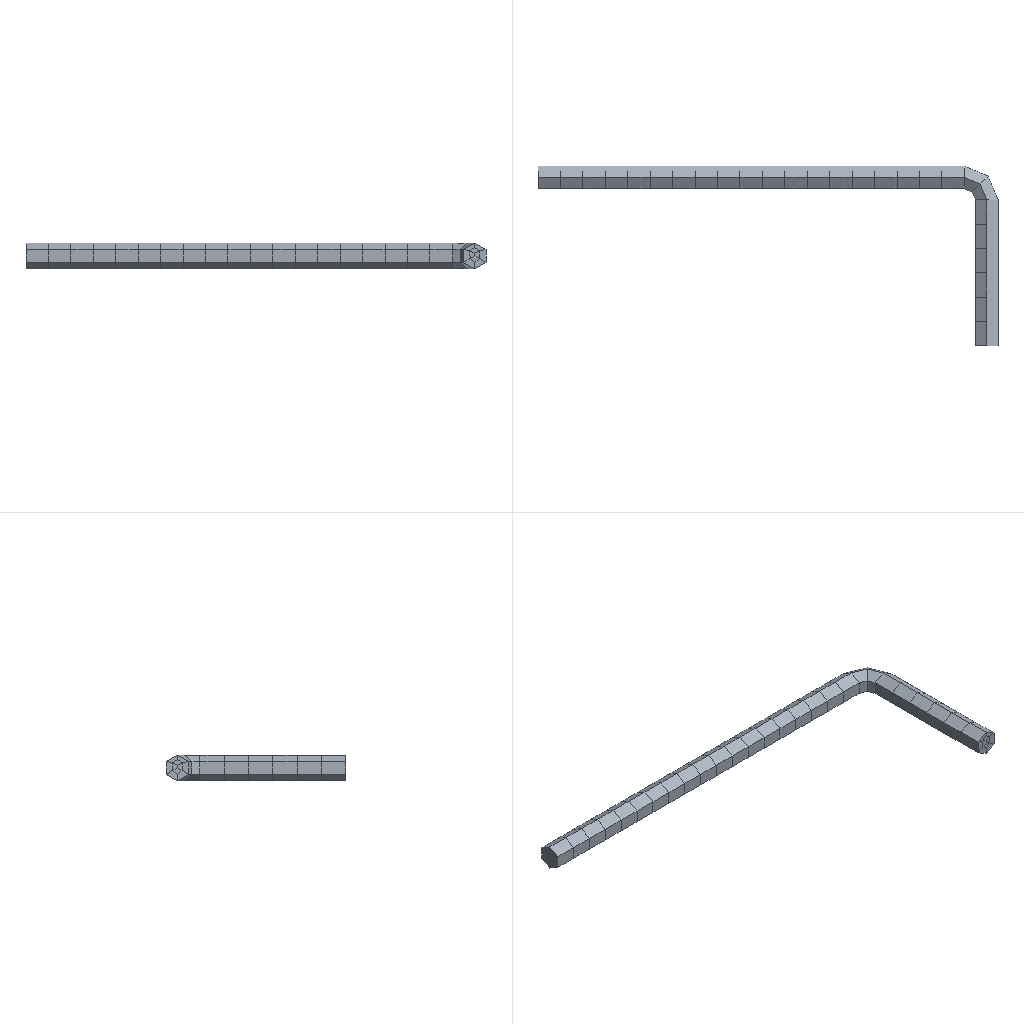Simulation study | ansys workbench
Ansys APDL input file, long lists of numbers shortened:
/batch
/config,noeldb,1     ! force off writing results to database
*get,_wallstrt,active,,time,wall
! ANSYS input file written by Workbench version 2022 R1
! File used for geometry attach:
/title,___--__ (C5)
! ****** Begin Custom Load Command Snippet ******
/COM, ACT Extensions:
/COM,     LSDYNA, 2021.1
/COM,
! ****** End   Custom Load Command Snippet ******
*DIM,_wb_ProjectScratch_dir,string,248
_wb_ProjectScratch_dir(1) = ''
*DIM,_wb_SolverFiles_dir,string,248
_wb_SolverFiles_dir(1) = ''
*DIM,_wb_userfiles_dir,string,248
_wb_userfiles_dir(1) = ''
/com,--- Data in consistent NMM units. See Solving Units in the help system for more information.
/units,MPA
/nopr
/wb,file,start              !  signify a WB generated input file
/prep7
! Turn off shape checking because checks already performed inside WB mesher.
! See help system for more information.
SHPP,OFF,,NOWARN
/nolist
etcon,set             ! allow ANSYS to choose best KEYOP's for 180x elements, resets any applicable keyopt to MAPDL defaults
/com,*********** Nodes for the whole assembly ***********
nblock,3,,1555
(1i9,3e20.9e3)
        1     1.000000000E+01     4.526588428E-02     2.653613818E-02
! (1413 more lines like these left out)
-1
/wb,elem,start            !  set before creation of elements
/com,*********** Elements for Body 1 "_____-FreeParts|__1" ***********
et,1,186
keyo,1,2,1          ! set full integration on SOLID186
eblock,19,solid,,270
(19i9)
        1        1        1        1        0        0        0        0       20        0        1        1        3        5        4      216      214      212      213
! (539 more lines like these left out)
-1
/wb,elem,end               !  done creating elements
/com,*********** Send User Defined Coordinate System(s) ***********
csys,0
toffst,273.15,  ! Temperature offset from absolute zero
/com,*********** Set Reference Temperature ***********
tref,22.
/wb,mat,start              !  starting to send materials
/com,*********** Send Materials ***********
Temperature = 'TEMP' ! Temperature
MP,DENS,1,7.85e-09,	! tonne mm^-3
MP,ALPX,1,1.2e-05,	! C^-1
MP,C,1,434000000,	! mm^2 s^-2 C^-1
MP,KXX,1,60.5,	! tonne mm s^-3 C^-1
MP,RSVX,1,0.00017,	! ohm mm
MP,EX,1,200000,	! tonne s^-2 mm^-1
MP,NUXY,1,0.3,
MP,MURX,1,10000,
/wb,mat,end                !  done sending materials
!************************* Model Summary ********************
!_____-FreeParts|__1,	结构钢,	matid,	1
!************************* End Model Summary ********************
! get the diagonal of the bounding box. Needed later for other things
*get,_xmin,node,,mnloc,x
*get,_ymin,node,,mnloc,y
*get,_zmin,node,,mnloc,z
*get,_xmax,node,,mxloc,x
*get,_ymax,node,,mxloc,y
*get,_zmax,node,,mxloc,z
_ASMDIAG=(_xmax-_xmin)*(_xmax-_xmin)+(_ymax-_ymin)*(_ymax-_ymin)+(_zmax-_zmin)*(_zmax-_zmin)
_ASMDIAG=SQRT(_ASMDIAG)
/wb,contact,start          !  starting to send contact
/wb,contact,end            !  done creating contacts
/golist
/wb,load,start             !  starting to send loads
/gst,on,on
fini
*get,_numnode,node,0,count
*get,_numelem,elem,0,count
*get, _MAXELEMNUM, elem, 0, NUM, MAX
*get, _MAXNODENUM, node, 0, NUM, MAX
*get, _MAXELEMTYPE, etyp, 0, NUM, MAX
*get, _MAXREALCONST, real, 0, NUM, MAX
/go
/wb,load,end               !  done creating loads
/com,--- Number of total nodes = %_numnode%
/com,--- Number of contact elements = 0
/com,--- Number of spring elements = 0
/com,--- Number of bearing elements = 0
/com,--- Number of solid elements = 270
/com,--- Number of condensed parts = 0
/com,--- Number of total elements = %_numelem%
*get,_wallbsol,active,,time,wall
/solu
antype,2                   ! modal analysis
_thickRatio=  1     ! Ratio of thick parts in the model
modopt,lanb,10
outres,erase
outres,all,none
outres,nsol,all
outres,etmp,all
mxpand                    ! default expand in case of complex solution
dmpopt,esav,no
dmpopt,emat,no
dmpopt,full,no
! *********** WB SOLVE COMMAND ***********
! check interactive state
*get,ANSINTER_,active,,int
*if,ANSINTER_,ne,0,then
/eof
*endif
solve
/com *************** Write FE CONNECTORS *********
CEWRITE,file,ce,,INTE
*get,_nmodalsolproc,active,0,numcpu
fini
/nopr
*get,_numnode,node,0,count
*get,_numelem,elem,0,count
*get, _MAXELEMNUM, elem, 0, NUM, MAX
*get, _MAXNODENUM, node, 0, NUM, MAX,,,INTERNAL
*get, _MAXELEMTYPE, etyp, 0, NUM, MAX
*get, _MAXREALCONST, real, 0, NUM, MAX
/gopr
*get,_wallasol,active,,time,wall
/post1
/nopr
*dim,_direction,CHAR,6,1
_direction(1) = 'X'
_direction(2) = 'Y'
_direction(3) = 'Z'
_direction(4) = 'ROTX'
_direction(5) = 'ROTY'
_direction(6) = 'ROTZ'
*get,_lastLS,active,0,set,LSTP
*get,_beginset,active,0,set,nset,first,_lastLS
*get,_endset,active,0,set,nset,last,_lastLS
_nummodes = 0
*if,_endset,gt,0,then
_nummodes = _endset - _beginset + 1
*endif
*do,i_mode,1,_nummodes
   *do,j_component,1,6
			*get,PFACT_%i_mode%_%j_component%,MODE,%i_mode%,PFACT,,DIREC,_direction(%j_component%)
   *enddo
*enddo
*dim,_tmdirection,CHAR,6,1
_tmdirection(1) = 'X'
_tmdirection(2) = 'Y'
_tmdirection(3) = 'Z'
_tmdirection(4) = 'X'
_tmdirection(5) = 'Y'
_tmdirection(6) = 'Z'
*do,j_component,1,6
    *if,j_component,gt,3,then
        *get,TOTALMASS_%j_component%,ELEM,0,IOR,_tmdirection(%j_component%)
    *else
        *get,TOTALMASS_%j_component%,ELEM,0,MTOT,_tmdirection(%j_component%)
    *endif
*enddo
/gopr
xmlo,ENCODING,ISO-8859-1
xmlo,parm
/xml,parm,xml
fini
/gopr
*get,_walldone,active,,time,wall
_preptime=(_wallbsol-_wallstrt)*3600
_solvtime=(_wallasol-_wallbsol)*3600
_posttime=(_walldone-_wallasol)*3600
_totaltim=(_walldone-_wallstrt)*3600
*get,_dlbratio,active,0,solu,dlbr
*get,_combtime,active,0,solu,comb
*get,_ssmode,active,0,solu,ssmm
*get,_ndofs,active,0,solu,ndof
/fclean				!clean distributed files
/com,--- Total number of nodes = %_numnode%
/com,--- Total number of elements = %_numelem%
/com,--- Element load balance ratio = %_dlbratio%
/com,--- Time to combine distributed files = %_combtime%
/com,--- Sparse memory mode = %_ssmode%
/com,--- Number of DOF = %_ndofs%
/wb,file,end               ! done with WB generated input